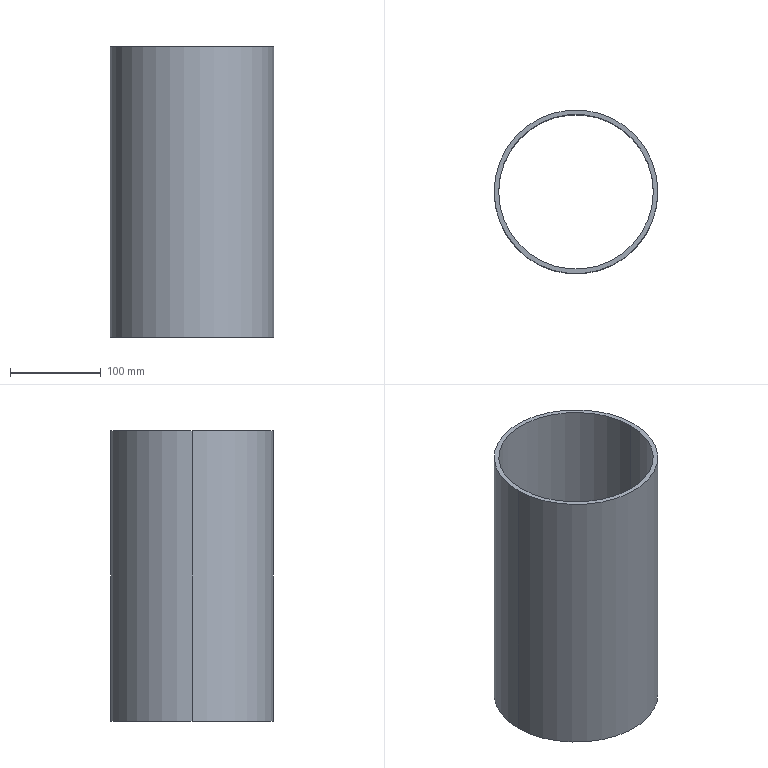Part | SolidWorks | features Extrusion 1 | 1 solid | 6 faces | box 180 x 180 x 320 mm | volume 879646 mm3 | cylinder 4 | plane 2 | commonest cylinder face diameters 170 x2 180 x2
STEP:
#1=CARTESIAN_POINT('',(-85.,0.,320.));
#2=VERTEX_POINT('',#1);
#3=CARTESIAN_POINT('',(85.,0.,320.));
#4=VERTEX_POINT('',#3);
#5=CARTESIAN_POINT('',(0.,0.,320.));
#6=DIRECTION('',(0.,0.,1.));
#7=DIRECTION('',(1.,0.,0.));
#8=AXIS2_PLACEMENT_3D('',#5,#6,#7);
#9=CIRCLE('',#8,85.);
#10=EDGE_CURVE('',#2,#4,#9,.T.);
#11=ORIENTED_EDGE('',*,*,#10,.T.);
#12=CARTESIAN_POINT('',(85.,0.,0.));
#13=VERTEX_POINT('',#12);
#14=CARTESIAN_POINT('',(85.,0.,320.));
#15=DIRECTION('',(0.,0.,-1.));
#16=VECTOR('',#15,1000.);
#17=LINE('',#14,#16);
#18=EDGE_CURVE('',#4,#13,#17,.T.);
#19=ORIENTED_EDGE('',*,*,#18,.T.);
#20=CARTESIAN_POINT('',(-85.,0.,0.));
#21=VERTEX_POINT('',#20);
#22=CARTESIAN_POINT('',(0.,0.,0.));
#23=DIRECTION('',(0.,0.,1.));
#24=DIRECTION('',(1.,0.,0.));
#25=AXIS2_PLACEMENT_3D('',#22,#23,#24);
#26=CIRCLE('',#25,85.);
#27=EDGE_CURVE('',#21,#13,#26,.T.);
#28=ORIENTED_EDGE('',*,*,#27,.F.);
#29=CARTESIAN_POINT('',(-85.,0.,320.));
#30=DIRECTION('',(0.,0.,-1.));
#31=VECTOR('',#30,1000.);
#32=LINE('',#29,#31);
#33=EDGE_CURVE('',#2,#21,#32,.T.);
#34=ORIENTED_EDGE('',*,*,#33,.F.);
#35=EDGE_LOOP('',(#11,#19,#28,#34));
#36=FACE_OUTER_BOUND('',#35,.T.);
#37=CARTESIAN_POINT('',(0.,0.,320.));
#38=DIRECTION('',(0.,0.,-1.));
#39=DIRECTION('',(-1.,0.,0.));
#40=AXIS2_PLACEMENT_3D('',#37,#38,#39);
#41=CYLINDRICAL_SURFACE('',#40,85.);
#42=ADVANCED_FACE('',(#36),#41,.F.);
#43=CARTESIAN_POINT('',(90.,0.,320.));
#44=VERTEX_POINT('',#43);
#45=CARTESIAN_POINT('',(-90.,0.,320.));
#46=VERTEX_POINT('',#45);
#47=CARTESIAN_POINT('',(0.,0.,320.));
#48=DIRECTION('',(0.,0.,1.));
#49=DIRECTION('',(1.,0.,0.));
#50=AXIS2_PLACEMENT_3D('',#47,#48,#49);
#51=CIRCLE('',#50,90.);
#52=EDGE_CURVE('',#44,#46,#51,.T.);
#53=ORIENTED_EDGE('',*,*,#52,.F.);
#54=CARTESIAN_POINT('',(90.,0.,0.));
#55=VERTEX_POINT('',#54);
#56=CARTESIAN_POINT('',(90.,0.,320.));
#57=DIRECTION('',(0.,0.,-1.));
#58=VECTOR('',#57,1000.);
#59=LINE('',#56,#58);
#60=EDGE_CURVE('',#44,#55,#59,.T.);
#61=ORIENTED_EDGE('',*,*,#60,.T.);
#62=CARTESIAN_POINT('',(-90.,0.,0.));
#63=VERTEX_POINT('',#62);
#64=CARTESIAN_POINT('',(0.,0.,0.));
#65=DIRECTION('',(0.,0.,1.));
#66=DIRECTION('',(1.,0.,0.));
#67=AXIS2_PLACEMENT_3D('',#64,#65,#66);
#68=CIRCLE('',#67,90.);
#69=EDGE_CURVE('',#55,#63,#68,.T.);
#70=ORIENTED_EDGE('',*,*,#69,.T.);
#71=CARTESIAN_POINT('',(-90.,0.,320.));
#72=DIRECTION('',(0.,0.,-1.));
#73=VECTOR('',#72,1000.);
#74=LINE('',#71,#73);
#75=EDGE_CURVE('',#46,#63,#74,.T.);
#76=ORIENTED_EDGE('',*,*,#75,.F.);
#77=EDGE_LOOP('',(#53,#61,#70,#76));
#78=FACE_OUTER_BOUND('',#77,.T.);
#79=CARTESIAN_POINT('',(0.,0.,320.));
#80=DIRECTION('',(0.,0.,-1.));
#81=DIRECTION('',(-1.,0.,0.));
#82=AXIS2_PLACEMENT_3D('',#79,#80,#81);
#83=CYLINDRICAL_SURFACE('',#82,90.);
#84=ADVANCED_FACE('',(#78),#83,.T.);
#85=CARTESIAN_POINT('',(0.,0.,320.));
#86=DIRECTION('',(0.,0.,1.));
#87=DIRECTION('',(1.,0.,0.));
#88=AXIS2_PLACEMENT_3D('',#85,#86,#87);
#89=CIRCLE('',#88,90.);
#90=EDGE_CURVE('',#46,#44,#89,.T.);
#91=ORIENTED_EDGE('',*,*,#90,.T.);
#92=ORIENTED_EDGE('',*,*,#52,.T.);
#93=EDGE_LOOP('',(#91,#92));
#94=FACE_OUTER_BOUND('',#93,.T.);
#95=ORIENTED_EDGE('',*,*,#10,.F.);
#96=CARTESIAN_POINT('',(0.,0.,320.));
#97=DIRECTION('',(0.,0.,1.));
#98=DIRECTION('',(1.,0.,0.));
#99=AXIS2_PLACEMENT_3D('',#96,#97,#98);
#100=CIRCLE('',#99,85.);
#101=EDGE_CURVE('',#4,#2,#100,.T.);
#102=ORIENTED_EDGE('',*,*,#101,.F.);
#103=EDGE_LOOP('',(#95,#102));
#104=FACE_BOUND('',#103,.T.);
#105=CARTESIAN_POINT('',(0.,0.,320.));
#106=DIRECTION('',(0.,0.,1.));
#107=DIRECTION('',(1.,0.,0.));
#108=AXIS2_PLACEMENT_3D('',#105,#106,#107);
#109=PLANE('',#108);
#110=ADVANCED_FACE('',(#94,#104),#109,.T.);
#111=CARTESIAN_POINT('',(0.,0.,0.));
#112=DIRECTION('',(0.,0.,1.));
#113=DIRECTION('',(1.,0.,0.));
#114=AXIS2_PLACEMENT_3D('',#111,#112,#113);
#115=CIRCLE('',#114,90.);
#116=EDGE_CURVE('',#63,#55,#115,.T.);
#117=ORIENTED_EDGE('',*,*,#116,.F.);
#118=ORIENTED_EDGE('',*,*,#69,.F.);
#119=EDGE_LOOP('',(#117,#118));
#120=FACE_OUTER_BOUND('',#119,.T.);
#121=ORIENTED_EDGE('',*,*,#27,.T.);
#122=CARTESIAN_POINT('',(0.,0.,0.));
#123=DIRECTION('',(0.,0.,1.));
#124=DIRECTION('',(1.,0.,0.));
#125=AXIS2_PLACEMENT_3D('',#122,#123,#124);
#126=CIRCLE('',#125,85.);
#127=EDGE_CURVE('',#13,#21,#126,.T.);
#128=ORIENTED_EDGE('',*,*,#127,.T.);
#129=EDGE_LOOP('',(#121,#128));
#130=FACE_BOUND('',#129,.T.);
#131=CARTESIAN_POINT('',(0.,0.,0.));
#132=DIRECTION('',(0.,0.,1.));
#133=DIRECTION('',(1.,0.,0.));
#134=AXIS2_PLACEMENT_3D('',#131,#132,#133);
#135=PLANE('',#134);
#136=ADVANCED_FACE('',(#120,#130),#135,.F.);
#137=ORIENTED_EDGE('',*,*,#60,.F.);
#138=ORIENTED_EDGE('',*,*,#90,.F.);
#139=ORIENTED_EDGE('',*,*,#75,.T.);
#140=ORIENTED_EDGE('',*,*,#116,.T.);
#141=EDGE_LOOP('',(#137,#138,#139,#140));
#142=FACE_OUTER_BOUND('',#141,.T.);
#143=CARTESIAN_POINT('',(0.,0.,320.));
#144=DIRECTION('',(0.,0.,-1.));
#145=DIRECTION('',(-1.,0.,0.));
#146=AXIS2_PLACEMENT_3D('',#143,#144,#145);
#147=CYLINDRICAL_SURFACE('',#146,90.);
#148=ADVANCED_FACE('',(#142),#147,.T.);
#149=ORIENTED_EDGE('',*,*,#18,.F.);
#150=ORIENTED_EDGE('',*,*,#101,.T.);
#151=ORIENTED_EDGE('',*,*,#33,.T.);
#152=ORIENTED_EDGE('',*,*,#127,.F.);
#153=EDGE_LOOP('',(#149,#150,#151,#152));
#154=FACE_OUTER_BOUND('',#153,.T.);
#155=CARTESIAN_POINT('',(0.,0.,320.));
#156=DIRECTION('',(0.,0.,-1.));
#157=DIRECTION('',(-1.,0.,0.));
#158=AXIS2_PLACEMENT_3D('',#155,#156,#157);
#159=CYLINDRICAL_SURFACE('',#158,85.);
#160=ADVANCED_FACE('',(#154),#159,.F.);
#161=CLOSED_SHELL('',(#42,#84,#110,#136,#148,#160));
#162=MANIFOLD_SOLID_BREP('',#161);
#163=CARTESIAN_POINT('',(0.,0.,0.));
#164=DIRECTION('',(0.,0.,1.));
#165=DIRECTION('',(1.,0.,0.));
#166=AXIS2_PLACEMENT_3D('',#163,#164,#165);
#167=(LENGTH_UNIT()NAMED_UNIT(*)SI_UNIT(.MILLI.,.METRE.));
#168=UNCERTAINTY_MEASURE_WITH_UNIT(LENGTH_MEASURE(0.00001),#167,'','');
#169=(NAMED_UNIT(*)PLANE_ANGLE_UNIT()SI_UNIT($,.RADIAN.));
#170=(NAMED_UNIT(*)SI_UNIT($,.STERADIAN.)SOLID_ANGLE_UNIT());
#171=(GEOMETRIC_REPRESENTATION_CONTEXT(3)GLOBAL_UNCERTAINTY_ASSIGNED_CONTEXT((#168))GLOBAL_UNIT_ASSIGNED_CONTEXT((#167,#169,#170))REPRESENTATION_CONTEXT('',''));
#172=ADVANCED_BREP_SHAPE_REPRESENTATION('',(#162,#166),#171);